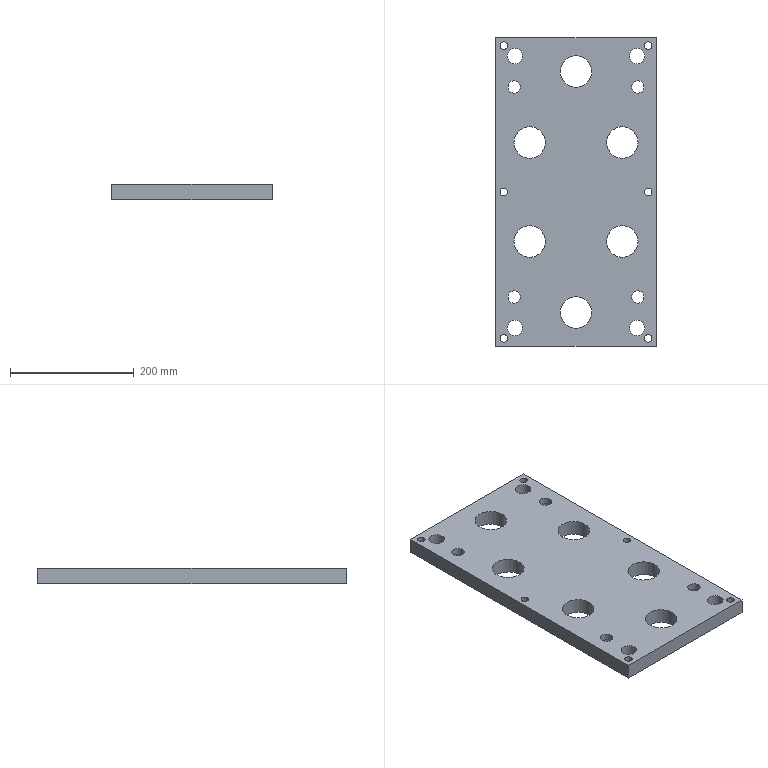Part | STEP file | SL2-MOLD_id702_xmt_txt | 1 solid | 42 faces | box 260 x 500 x 25 mm | volume 2824522 mm3 | cylinder 28 | plane 14 | commonest cylinder face diameters 12 x6 51 x6 20 x4 25 x4 28.5 x4 30 x4
STEP:
#1=CARTESIAN_POINT('',(49.5,170.,-214.));
#2=VERTEX_POINT('',#1);
#3=CARTESIAN_POINT('',(75.,170.,-214.));
#4=DIRECTION('',(0.,0.,-1.));
#5=DIRECTION('',(-1.,0.,0.));
#6=AXIS2_PLACEMENT_3D('',#3,#4,#5);
#7=CIRCLE('',#6,25.5);
#8=EDGE_CURVE('',#2,#2,#7,.T.);
#9=ORIENTED_EDGE('',*,*,#8,.F.);
#10=EDGE_LOOP('',(#9));
#11=FACE_BOUND('',#10,.T.);
#12=CARTESIAN_POINT('',(49.5,10.,-214.));
#13=VERTEX_POINT('',#12);
#14=CARTESIAN_POINT('',(75.,10.,-214.));
#15=DIRECTION('',(0.,0.,-1.));
#16=DIRECTION('',(-1.,0.,0.));
#17=AXIS2_PLACEMENT_3D('',#14,#15,#16);
#18=CIRCLE('',#17,25.5);
#19=EDGE_CURVE('',#13,#13,#18,.T.);
#20=ORIENTED_EDGE('',*,*,#19,.F.);
#21=EDGE_LOOP('',(#20));
#22=FACE_BOUND('',#21,.T.);
#23=CARTESIAN_POINT('',(-25.5,285.,-214.));
#24=VERTEX_POINT('',#23);
#25=CARTESIAN_POINT('',(0.,285.,-214.));
#26=DIRECTION('',(0.,0.,-1.));
#27=DIRECTION('',(-1.,0.,0.));
#28=AXIS2_PLACEMENT_3D('',#25,#26,#27);
#29=CIRCLE('',#28,25.5);
#30=EDGE_CURVE('',#24,#24,#29,.T.);
#31=ORIENTED_EDGE('',*,*,#30,.F.);
#32=EDGE_LOOP('',(#31));
#33=FACE_BOUND('',#32,.T.);
#34=CARTESIAN_POINT('',(-100.5,170.,-214.));
#35=VERTEX_POINT('',#34);
#36=CARTESIAN_POINT('',(-75.,170.,-214.));
#37=DIRECTION('',(0.,0.,-1.));
#38=DIRECTION('',(-1.,0.,0.));
#39=AXIS2_PLACEMENT_3D('',#36,#37,#38);
#40=CIRCLE('',#39,25.5);
#41=EDGE_CURVE('',#35,#35,#40,.T.);
#42=ORIENTED_EDGE('',*,*,#41,.F.);
#43=EDGE_LOOP('',(#42));
#44=FACE_BOUND('',#43,.T.);
#45=CARTESIAN_POINT('',(-25.5,-105.,-214.));
#46=VERTEX_POINT('',#45);
#47=CARTESIAN_POINT('',(0.,-105.,-214.));
#48=DIRECTION('',(0.,0.,-1.));
#49=DIRECTION('',(-1.,0.,0.));
#50=AXIS2_PLACEMENT_3D('',#47,#48,#49);
#51=CIRCLE('',#50,25.5);
#52=EDGE_CURVE('',#46,#46,#51,.T.);
#53=ORIENTED_EDGE('',*,*,#52,.F.);
#54=EDGE_LOOP('',(#53));
#55=FACE_BOUND('',#54,.T.);
#56=CARTESIAN_POINT('',(-100.5,10.,-214.));
#57=VERTEX_POINT('',#56);
#58=CARTESIAN_POINT('',(-75.,10.,-214.));
#59=DIRECTION('',(0.,0.,-1.));
#60=DIRECTION('',(-1.,0.,0.));
#61=AXIS2_PLACEMENT_3D('',#58,#59,#60);
#62=CIRCLE('',#61,25.5);
#63=EDGE_CURVE('',#57,#57,#62,.T.);
#64=ORIENTED_EDGE('',*,*,#63,.F.);
#65=EDGE_LOOP('',(#64));
#66=FACE_BOUND('',#65,.T.);
#67=CARTESIAN_POINT('',(-114.25,-80.,-214.));
#68=VERTEX_POINT('',#67);
#69=CARTESIAN_POINT('',(-100.,-80.,-214.));
#70=DIRECTION('',(0.,0.,1.));
#71=DIRECTION('',(-1.,0.,0.));
#72=AXIS2_PLACEMENT_3D('',#69,#70,#71);
#73=CIRCLE('',#72,14.25);
#74=EDGE_CURVE('',#68,#68,#73,.T.);
#75=ORIENTED_EDGE('',*,*,#74,.T.);
#76=EDGE_LOOP('',(#75));
#77=FACE_BOUND('',#76,.T.);
#78=CARTESIAN_POINT('',(85.75,-80.,-214.));
#79=VERTEX_POINT('',#78);
#80=CARTESIAN_POINT('',(100.,-80.,-214.));
#81=DIRECTION('',(0.,0.,1.));
#82=DIRECTION('',(-1.,0.,0.));
#83=AXIS2_PLACEMENT_3D('',#80,#81,#82);
#84=CIRCLE('',#83,14.25);
#85=EDGE_CURVE('',#79,#79,#84,.T.);
#86=ORIENTED_EDGE('',*,*,#85,.T.);
#87=EDGE_LOOP('',(#86));
#88=FACE_BOUND('',#87,.T.);
#89=CARTESIAN_POINT('',(85.75,260.,-214.));
#90=VERTEX_POINT('',#89);
#91=CARTESIAN_POINT('',(100.,260.,-214.));
#92=DIRECTION('',(0.,0.,1.));
#93=DIRECTION('',(-1.,0.,0.));
#94=AXIS2_PLACEMENT_3D('',#91,#92,#93);
#95=CIRCLE('',#94,14.25);
#96=EDGE_CURVE('',#90,#90,#95,.T.);
#97=ORIENTED_EDGE('',*,*,#96,.T.);
#98=EDGE_LOOP('',(#97));
#99=FACE_BOUND('',#98,.T.);
#100=CARTESIAN_POINT('',(-114.25,260.,-214.));
#101=VERTEX_POINT('',#100);
#102=CARTESIAN_POINT('',(-100.,260.,-214.));
#103=DIRECTION('',(0.,0.,1.));
#104=DIRECTION('',(-1.,0.,0.));
#105=AXIS2_PLACEMENT_3D('',#102,#103,#104);
#106=CIRCLE('',#105,14.25);
#107=EDGE_CURVE('',#101,#101,#106,.T.);
#108=ORIENTED_EDGE('',*,*,#107,.T.);
#109=EDGE_LOOP('',(#108));
#110=FACE_BOUND('',#109,.T.);
#111=CARTESIAN_POINT('',(-114.,310.,-214.));
#112=VERTEX_POINT('',#111);
#113=CARTESIAN_POINT('',(-99.,310.,-214.));
#114=DIRECTION('',(0.,0.,1.));
#115=DIRECTION('',(-1.,0.,0.));
#116=AXIS2_PLACEMENT_3D('',#113,#114,#115);
#117=CIRCLE('',#116,15.);
#118=EDGE_CURVE('',#112,#112,#117,.T.);
#119=ORIENTED_EDGE('',*,*,#118,.T.);
#120=EDGE_LOOP('',(#119));
#121=FACE_BOUND('',#120,.T.);
#122=CARTESIAN_POINT('',(84.,310.,-214.));
#123=VERTEX_POINT('',#122);
#124=CARTESIAN_POINT('',(99.,310.,-214.));
#125=DIRECTION('',(0.,0.,1.));
#126=DIRECTION('',(-1.,0.,0.));
#127=AXIS2_PLACEMENT_3D('',#124,#125,#126);
#128=CIRCLE('',#127,15.);
#129=EDGE_CURVE('',#123,#123,#128,.T.);
#130=ORIENTED_EDGE('',*,*,#129,.T.);
#131=EDGE_LOOP('',(#130));
#132=FACE_BOUND('',#131,.T.);
#133=CARTESIAN_POINT('',(84.,-130.,-214.));
#134=VERTEX_POINT('',#133);
#135=CARTESIAN_POINT('',(99.,-130.,-214.));
#136=DIRECTION('',(0.,0.,1.));
#137=DIRECTION('',(-1.,0.,0.));
#138=AXIS2_PLACEMENT_3D('',#135,#136,#137);
#139=CIRCLE('',#138,15.);
#140=EDGE_CURVE('',#134,#134,#139,.T.);
#141=ORIENTED_EDGE('',*,*,#140,.T.);
#142=EDGE_LOOP('',(#141));
#143=FACE_BOUND('',#142,.T.);
#144=CARTESIAN_POINT('',(-114.,-130.,-214.));
#145=VERTEX_POINT('',#144);
#146=CARTESIAN_POINT('',(-99.,-130.,-214.));
#147=DIRECTION('',(0.,0.,1.));
#148=DIRECTION('',(-1.,0.,0.));
#149=AXIS2_PLACEMENT_3D('',#146,#147,#148);
#150=CIRCLE('',#149,15.);
#151=EDGE_CURVE('',#145,#145,#150,.T.);
#152=ORIENTED_EDGE('',*,*,#151,.T.);
#153=EDGE_LOOP('',(#152));
#154=FACE_BOUND('',#153,.T.);
#155=CARTESIAN_POINT('',(111.,-147.,-214.));
#156=VERTEX_POINT('',#155);
#157=CARTESIAN_POINT('',(117.,-147.,-214.));
#158=DIRECTION('',(0.,0.,-1.));
#159=DIRECTION('',(-1.,0.,0.));
#160=AXIS2_PLACEMENT_3D('',#157,#158,#159);
#161=CIRCLE('',#160,6.);
#162=EDGE_CURVE('',#156,#156,#161,.T.);
#163=ORIENTED_EDGE('',*,*,#162,.F.);
#164=EDGE_LOOP('',(#163));
#165=FACE_BOUND('',#164,.T.);
#166=CARTESIAN_POINT('',(-123.,327.,-214.));
#167=VERTEX_POINT('',#166);
#168=CARTESIAN_POINT('',(-117.,327.,-214.));
#169=DIRECTION('',(0.,0.,-1.));
#170=DIRECTION('',(-1.,0.,0.));
#171=AXIS2_PLACEMENT_3D('',#168,#169,#170);
#172=CIRCLE('',#171,6.);
#173=EDGE_CURVE('',#167,#167,#172,.T.);
#174=ORIENTED_EDGE('',*,*,#173,.F.);
#175=EDGE_LOOP('',(#174));
#176=FACE_BOUND('',#175,.T.);
#177=CARTESIAN_POINT('',(-123.,-147.,-214.));
#178=VERTEX_POINT('',#177);
#179=CARTESIAN_POINT('',(-117.,-147.,-214.));
#180=DIRECTION('',(0.,0.,-1.));
#181=DIRECTION('',(-1.,0.,0.));
#182=AXIS2_PLACEMENT_3D('',#179,#180,#181);
#183=CIRCLE('',#182,6.);
#184=EDGE_CURVE('',#178,#178,#183,.T.);
#185=ORIENTED_EDGE('',*,*,#184,.F.);
#186=EDGE_LOOP('',(#185));
#187=FACE_BOUND('',#186,.T.);
#188=CARTESIAN_POINT('',(-123.,90.,-214.));
#189=VERTEX_POINT('',#188);
#190=CARTESIAN_POINT('',(-117.,90.,-214.));
#191=DIRECTION('',(0.,0.,-1.));
#192=DIRECTION('',(-1.,0.,0.));
#193=AXIS2_PLACEMENT_3D('',#190,#191,#192);
#194=CIRCLE('',#193,6.);
#195=EDGE_CURVE('',#189,#189,#194,.T.);
#196=ORIENTED_EDGE('',*,*,#195,.F.);
#197=EDGE_LOOP('',(#196));
#198=FACE_BOUND('',#197,.T.);
#199=CARTESIAN_POINT('',(111.,327.,-214.));
#200=VERTEX_POINT('',#199);
#201=CARTESIAN_POINT('',(117.,327.,-214.));
#202=DIRECTION('',(0.,0.,-1.));
#203=DIRECTION('',(-1.,0.,0.));
#204=AXIS2_PLACEMENT_3D('',#201,#202,#203);
#205=CIRCLE('',#204,6.);
#206=EDGE_CURVE('',#200,#200,#205,.T.);
#207=ORIENTED_EDGE('',*,*,#206,.F.);
#208=EDGE_LOOP('',(#207));
#209=FACE_BOUND('',#208,.T.);
#210=CARTESIAN_POINT('',(111.,90.,-214.));
#211=VERTEX_POINT('',#210);
#212=CARTESIAN_POINT('',(117.,90.,-214.));
#213=DIRECTION('',(0.,0.,-1.));
#214=DIRECTION('',(-1.,0.,0.));
#215=AXIS2_PLACEMENT_3D('',#212,#213,#214);
#216=CIRCLE('',#215,6.);
#217=EDGE_CURVE('',#211,#211,#216,.T.);
#218=ORIENTED_EDGE('',*,*,#217,.F.);
#219=EDGE_LOOP('',(#218));
#220=FACE_BOUND('',#219,.T.);
#221=CARTESIAN_POINT('',(-130.,-160.,-214.));
#222=VERTEX_POINT('',#221);
#223=CARTESIAN_POINT('',(130.,-160.,-214.));
#224=VERTEX_POINT('',#223);
#225=CARTESIAN_POINT('',(0.,-160.,-214.));
#226=DIRECTION('',(1.,0.,0.));
#227=VECTOR('',#226,1.);
#228=LINE('',#225,#227);
#229=EDGE_CURVE('',#222,#224,#228,.T.);
#230=ORIENTED_EDGE('',*,*,#229,.F.);
#231=CARTESIAN_POINT('',(-130.,340.,-214.));
#232=VERTEX_POINT('',#231);
#233=CARTESIAN_POINT('',(-130.,90.,-214.));
#234=DIRECTION('',(0.,1.,0.));
#235=VECTOR('',#234,1.);
#236=LINE('',#233,#235);
#237=EDGE_CURVE('',#222,#232,#236,.T.);
#238=ORIENTED_EDGE('',*,*,#237,.T.);
#239=CARTESIAN_POINT('',(130.,340.,-214.));
#240=VERTEX_POINT('',#239);
#241=CARTESIAN_POINT('',(0.,340.,-214.));
#242=DIRECTION('',(-1.,0.,0.));
#243=VECTOR('',#242,1.);
#244=LINE('',#241,#243);
#245=EDGE_CURVE('',#240,#232,#244,.T.);
#246=ORIENTED_EDGE('',*,*,#245,.F.);
#247=CARTESIAN_POINT('',(130.,90.,-214.));
#248=DIRECTION('',(0.,1.,0.));
#249=VECTOR('',#248,1.);
#250=LINE('',#247,#249);
#251=EDGE_CURVE('',#224,#240,#250,.T.);
#252=ORIENTED_EDGE('',*,*,#251,.F.);
#253=EDGE_LOOP('',(#230,#238,#246,#252));
#254=FACE_BOUND('',#253,.T.);
#255=CARTESIAN_POINT('',(0.,90.,-214.));
#256=DIRECTION('',(0.,0.,-1.));
#257=DIRECTION('',(-1.,0.,0.));
#258=AXIS2_PLACEMENT_3D('',#255,#256,#257);
#259=PLANE('',#258);
#260=ADVANCED_FACE('',(#11,#22,#33,#44,#55,#66,#77,#88,#99,#110,#121,#132,#143,#154,#165,#176,#187,#198,#209,#220,#254),#259,.T.);
#261=CARTESIAN_POINT('',(-130.,340.,-189.));
#262=VERTEX_POINT('',#261);
#263=CARTESIAN_POINT('',(130.,340.,-189.));
#264=VERTEX_POINT('',#263);
#265=CARTESIAN_POINT('',(0.,340.,-189.));
#266=DIRECTION('',(1.,0.,0.));
#267=VECTOR('',#266,1.);
#268=LINE('',#265,#267);
#269=EDGE_CURVE('',#262,#264,#268,.T.);
#270=ORIENTED_EDGE('',*,*,#269,.T.);
#271=CARTESIAN_POINT('',(130.,340.,-244.));
#272=DIRECTION('',(0.,0.,-1.));
#273=VECTOR('',#272,1.);
#274=LINE('',#271,#273);
#275=EDGE_CURVE('',#264,#240,#274,.T.);
#276=ORIENTED_EDGE('',*,*,#275,.T.);
#277=ORIENTED_EDGE('',*,*,#245,.T.);
#278=CARTESIAN_POINT('',(-130.,340.,-244.));
#279=DIRECTION('',(0.,0.,1.));
#280=VECTOR('',#279,1.);
#281=LINE('',#278,#280);
#282=EDGE_CURVE('',#232,#262,#281,.T.);
#283=ORIENTED_EDGE('',*,*,#282,.T.);
#284=EDGE_LOOP('',(#270,#276,#277,#283));
#285=FACE_OUTER_BOUND('',#284,.T.);
#286=CARTESIAN_POINT('',(0.,340.,-244.));
#287=DIRECTION('',(0.,1.,0.));
#288=DIRECTION('',(0.,0.,1.));
#289=AXIS2_PLACEMENT_3D('',#286,#287,#288);
#290=PLANE('',#289);
#291=ADVANCED_FACE('',(#285),#290,.T.);
#292=CARTESIAN_POINT('',(-130.,-160.,-189.));
#293=VERTEX_POINT('',#292);
#294=CARTESIAN_POINT('',(130.,-160.,-189.));
#295=VERTEX_POINT('',#294);
#296=CARTESIAN_POINT('',(0.,-160.,-189.));
#297=DIRECTION('',(1.,0.,0.));
#298=VECTOR('',#297,1.);
#299=LINE('',#296,#298);
#300=EDGE_CURVE('',#293,#295,#299,.T.);
#301=ORIENTED_EDGE('',*,*,#300,.F.);
#302=CARTESIAN_POINT('',(-130.,-160.,-244.));
#303=DIRECTION('',(0.,0.,-1.));
#304=VECTOR('',#303,1.);
#305=LINE('',#302,#304);
#306=EDGE_CURVE('',#293,#222,#305,.T.);
#307=ORIENTED_EDGE('',*,*,#306,.T.);
#308=ORIENTED_EDGE('',*,*,#229,.T.);
#309=CARTESIAN_POINT('',(130.,-160.,-179.));
#310=DIRECTION('',(0.,0.,-1.));
#311=VECTOR('',#310,1.);
#312=LINE('',#309,#311);
#313=EDGE_CURVE('',#295,#224,#312,.T.);
#314=ORIENTED_EDGE('',*,*,#313,.F.);
#315=EDGE_LOOP('',(#301,#307,#308,#314));
#316=FACE_OUTER_BOUND('',#315,.T.);
#317=CARTESIAN_POINT('',(0.,-160.,-244.));
#318=DIRECTION('',(0.,-1.,0.));
#319=DIRECTION('',(0.,0.,-1.));
#320=AXIS2_PLACEMENT_3D('',#317,#318,#319);
#321=PLANE('',#320);
#322=ADVANCED_FACE('',(#316),#321,.T.);
#323=CARTESIAN_POINT('',(130.,90.,-189.));
#324=DIRECTION('',(0.,1.,0.));
#325=VECTOR('',#324,1.);
#326=LINE('',#323,#325);
#327=EDGE_CURVE('',#295,#264,#326,.T.);
#328=ORIENTED_EDGE('',*,*,#327,.F.);
#329=ORIENTED_EDGE('',*,*,#313,.T.);
#330=ORIENTED_EDGE('',*,*,#251,.T.);
#331=ORIENTED_EDGE('',*,*,#275,.F.);
#332=EDGE_LOOP('',(#328,#329,#330,#331));
#333=FACE_OUTER_BOUND('',#332,.T.);
#334=CARTESIAN_POINT('',(130.,90.,-179.));
#335=DIRECTION('',(1.,0.,0.));
#336=DIRECTION('',(0.,0.,-1.));
#337=AXIS2_PLACEMENT_3D('',#334,#335,#336);
#338=PLANE('',#337);
#339=ADVANCED_FACE('',(#333),#338,.T.);
#340=CARTESIAN_POINT('',(-130.,90.,-189.));
#341=DIRECTION('',(0.,-1.,0.));
#342=VECTOR('',#341,1.);
#343=LINE('',#340,#342);
#344=EDGE_CURVE('',#262,#293,#343,.T.);
#345=ORIENTED_EDGE('',*,*,#344,.F.);
#346=ORIENTED_EDGE('',*,*,#282,.F.);
#347=ORIENTED_EDGE('',*,*,#237,.F.);
#348=ORIENTED_EDGE('',*,*,#306,.F.);
#349=EDGE_LOOP('',(#345,#346,#347,#348));
#350=FACE_OUTER_BOUND('',#349,.T.);
#351=CARTESIAN_POINT('',(-130.,90.,-179.));
#352=DIRECTION('',(-1.,0.,0.));
#353=DIRECTION('',(0.,0.,1.));
#354=AXIS2_PLACEMENT_3D('',#351,#352,#353);
#355=PLANE('',#354);
#356=ADVANCED_FACE('',(#350),#355,.T.);
#357=CARTESIAN_POINT('',(49.5,170.,-189.));
#358=VERTEX_POINT('',#357);
#359=CARTESIAN_POINT('',(75.,170.,-189.));
#360=DIRECTION('',(0.,0.,-1.));
#361=DIRECTION('',(-1.,0.,0.));
#362=AXIS2_PLACEMENT_3D('',#359,#360,#361);
#363=CIRCLE('',#362,25.5);
#364=EDGE_CURVE('',#358,#358,#363,.T.);
#365=ORIENTED_EDGE('',*,*,#364,.T.);
#366=EDGE_LOOP('',(#365));
#367=FACE_BOUND('',#366,.T.);
#368=CARTESIAN_POINT('',(49.5,10.,-189.));
#369=VERTEX_POINT('',#368);
#370=CARTESIAN_POINT('',(75.,10.,-189.));
#371=DIRECTION('',(0.,0.,-1.));
#372=DIRECTION('',(-1.,0.,0.));
#373=AXIS2_PLACEMENT_3D('',#370,#371,#372);
#374=CIRCLE('',#373,25.5);
#375=EDGE_CURVE('',#369,#369,#374,.T.);
#376=ORIENTED_EDGE('',*,*,#375,.T.);
#377=EDGE_LOOP('',(#376));
#378=FACE_BOUND('',#377,.T.);
#379=CARTESIAN_POINT('',(-25.5,285.,-189.));
#380=VERTEX_POINT('',#379);
#381=CARTESIAN_POINT('',(0.,285.,-189.));
#382=DIRECTION('',(0.,0.,-1.));
#383=DIRECTION('',(-1.,0.,0.));
#384=AXIS2_PLACEMENT_3D('',#381,#382,#383);
#385=CIRCLE('',#384,25.5);
#386=EDGE_CURVE('',#380,#380,#385,.T.);
#387=ORIENTED_EDGE('',*,*,#386,.T.);
#388=EDGE_LOOP('',(#387));
#389=FACE_BOUND('',#388,.T.);
#390=CARTESIAN_POINT('',(-100.5,170.,-189.));
#391=VERTEX_POINT('',#390);
#392=CARTESIAN_POINT('',(-75.,170.,-189.));
#393=DIRECTION('',(0.,0.,-1.));
#394=DIRECTION('',(-1.,0.,0.));
#395=AXIS2_PLACEMENT_3D('',#392,#393,#394);
#396=CIRCLE('',#395,25.5);
#397=EDGE_CURVE('',#391,#391,#396,.T.);
#398=ORIENTED_EDGE('',*,*,#397,.T.);
#399=EDGE_LOOP('',(#398));
#400=FACE_BOUND('',#399,.T.);
#401=CARTESIAN_POINT('',(-25.5,-105.,-189.));
#402=VERTEX_POINT('',#401);
#403=CARTESIAN_POINT('',(0.,-105.,-189.));
#404=DIRECTION('',(0.,0.,-1.));
#405=DIRECTION('',(-1.,0.,0.));
#406=AXIS2_PLACEMENT_3D('',#403,#404,#405);
#407=CIRCLE('',#406,25.5);
#408=EDGE_CURVE('',#402,#402,#407,.T.);
#409=ORIENTED_EDGE('',*,*,#408,.T.);
#410=EDGE_LOOP('',(#409));
#411=FACE_BOUND('',#410,.T.);
#412=CARTESIAN_POINT('',(-100.5,10.,-189.));
#413=VERTEX_POINT('',#412);
#414=CARTESIAN_POINT('',(-75.,10.,-189.));
#415=DIRECTION('',(0.,0.,-1.));
#416=DIRECTION('',(-1.,0.,0.));
#417=AXIS2_PLACEMENT_3D('',#414,#415,#416);
#418=CIRCLE('',#417,25.5);
#419=EDGE_CURVE('',#413,#413,#418,.T.);
#420=ORIENTED_EDGE('',*,*,#419,.T.);
#421=EDGE_LOOP('',(#420));
#422=FACE_BOUND('',#421,.T.);
#423=CARTESIAN_POINT('',(90.,260.,-189.));
#424=VERTEX_POINT('',#423);
#425=CARTESIAN_POINT('',(100.,260.,-189.));
#426=DIRECTION('',(0.,0.,1.));
#427=DIRECTION('',(-1.,0.,0.));
#428=AXIS2_PLACEMENT_3D('',#425,#426,#427);
#429=CIRCLE('',#428,10.);
#430=EDGE_CURVE('',#424,#424,#429,.T.);
#431=ORIENTED_EDGE('',*,*,#430,.F.);
#432=EDGE_LOOP('',(#431));
#433=FACE_BOUND('',#432,.T.);
#434=CARTESIAN_POINT('',(90.,-80.,-189.));
#435=VERTEX_POINT('',#434);
#436=CARTESIAN_POINT('',(100.,-80.,-189.));
#437=DIRECTION('',(0.,0.,1.));
#438=DIRECTION('',(-1.,0.,0.));
#439=AXIS2_PLACEMENT_3D('',#436,#437,#438);
#440=CIRCLE('',#439,10.);
#441=EDGE_CURVE('',#435,#435,#440,.T.);
#442=ORIENTED_EDGE('',*,*,#441,.F.);
#443=EDGE_LOOP('',(#442));
#444=FACE_BOUND('',#443,.T.);
#445=CARTESIAN_POINT('',(-110.,-80.,-189.));
#446=VERTEX_POINT('',#445);
#447=CARTESIAN_POINT('',(-100.,-80.,-189.));
#448=DIRECTION('',(0.,0.,1.));
#449=DIRECTION('',(-1.,0.,0.));
#450=AXIS2_PLACEMENT_3D('',#447,#448,#449);
#451=CIRCLE('',#450,10.);
#452=EDGE_CURVE('',#446,#446,#451,.T.);
#453=ORIENTED_EDGE('',*,*,#452,.F.);
#454=EDGE_LOOP('',(#453));
#455=FACE_BOUND('',#454,.T.);
#456=CARTESIAN_POINT('',(-110.,260.,-189.));
#457=VERTEX_POINT('',#456);
#458=CARTESIAN_POINT('',(-100.,260.,-189.));
#459=DIRECTION('',(0.,0.,1.));
#460=DIRECTION('',(-1.,0.,0.));
#461=AXIS2_PLACEMENT_3D('',#458,#459,#460);
#462=CIRCLE('',#461,10.);
#463=EDGE_CURVE('',#457,#457,#462,.T.);
#464=ORIENTED_EDGE('',*,*,#463,.F.);
#465=EDGE_LOOP('',(#464));
#466=FACE_BOUND('',#465,.T.);
#467=CARTESIAN_POINT('',(86.5,310.,-189.));
#468=VERTEX_POINT('',#467);
#469=CARTESIAN_POINT('',(99.,310.,-189.));
#470=DIRECTION('',(0.,0.,1.));
#471=DIRECTION('',(-1.,0.,0.));
#472=AXIS2_PLACEMENT_3D('',#469,#470,#471);
#473=CIRCLE('',#472,12.5);
#474=EDGE_CURVE('',#468,#468,#473,.T.);
#475=ORIENTED_EDGE('',*,*,#474,.F.);
#476=EDGE_LOOP('',(#475));
#477=FACE_BOUND('',#476,.T.);
#478=CARTESIAN_POINT('',(-111.5,310.,-189.));
#479=VERTEX_POINT('',#478);
#480=CARTESIAN_POINT('',(-99.,310.,-189.));
#481=DIRECTION('',(0.,0.,1.));
#482=DIRECTION('',(-1.,0.,0.));
#483=AXIS2_PLACEMENT_3D('',#480,#481,#482);
#484=CIRCLE('',#483,12.5);
#485=EDGE_CURVE('',#479,#479,#484,.T.);
#486=ORIENTED_EDGE('',*,*,#485,.F.);
#487=EDGE_LOOP('',(#486));
#488=FACE_BOUND('',#487,.T.);
#489=CARTESIAN_POINT('',(86.5,-130.,-189.));
#490=VERTEX_POINT('',#489);
#491=CARTESIAN_POINT('',(99.,-130.,-189.));
#492=DIRECTION('',(0.,0.,1.));
#493=DIRECTION('',(-1.,0.,0.));
#494=AXIS2_PLACEMENT_3D('',#491,#492,#493);
#495=CIRCLE('',#494,12.5);
#496=EDGE_CURVE('',#490,#490,#495,.T.);
#497=ORIENTED_EDGE('',*,*,#496,.F.);
#498=EDGE_LOOP('',(#497));
#499=FACE_BOUND('',#498,.T.);
#500=CARTESIAN_POINT('',(-111.5,-130.,-189.));
#501=VERTEX_POINT('',#500);
#502=CARTESIAN_POINT('',(-99.,-130.,-189.));
#503=DIRECTION('',(0.,0.,1.));
#504=DIRECTION('',(-1.,0.,0.));
#505=AXIS2_PLACEMENT_3D('',#502,#503,#504);
#506=CIRCLE('',#505,12.5);
#507=EDGE_CURVE('',#501,#501,#506,.T.);
#508=ORIENTED_EDGE('',*,*,#507,.F.);
#509=EDGE_LOOP('',(#508));
#510=FACE_BOUND('',#509,.T.);
#511=CARTESIAN_POINT('',(111.,-147.,-189.));
#512=VERTEX_POINT('',#511);
#513=CARTESIAN_POINT('',(117.,-147.,-189.));
#514=DIRECTION('',(0.,0.,-1.));
#515=DIRECTION('',(-1.,0.,0.));
#516=AXIS2_PLACEMENT_3D('',#513,#514,#515);
#517=CIRCLE('',#516,6.);
#518=EDGE_CURVE('',#512,#512,#517,.T.);
#519=ORIENTED_EDGE('',*,*,#518,.T.);
#520=EDGE_LOOP('',(#519));
#521=FACE_BOUND('',#520,.T.);
#522=CARTESIAN_POINT('',(-123.,327.,-189.));
#523=VERTEX_POINT('',#522);
#524=CARTESIAN_POINT('',(-117.,327.,-189.));
#525=DIRECTION('',(0.,0.,-1.));
#526=DIRECTION('',(-1.,0.,0.));
#527=AXIS2_PLACEMENT_3D('',#524,#525,#526);
#528=CIRCLE('',#527,6.);
#529=EDGE_CURVE('',#523,#523,#528,.T.);
#530=ORIENTED_EDGE('',*,*,#529,.T.);
#531=EDGE_LOOP('',(#530));
#532=FACE_BOUND('',#531,.T.);
#533=CARTESIAN_POINT('',(-123.,-147.,-189.));
#534=VERTEX_POINT('',#533);
#535=CARTESIAN_POINT('',(-117.,-147.,-189.));
#536=DIRECTION('',(0.,0.,-1.));
#537=DIRECTION('',(-1.,0.,0.));
#538=AXIS2_PLACEMENT_3D('',#535,#536,#537);
#539=CIRCLE('',#538,6.);
#540=EDGE_CURVE('',#534,#534,#539,.T.);
#541=ORIENTED_EDGE('',*,*,#540,.T.);
#542=EDGE_LOOP('',(#541));
#543=FACE_BOUND('',#542,.T.);
#544=CARTESIAN_POINT('',(-123.,90.,-189.));
#545=VERTEX_POINT('',#544);
#546=CARTESIAN_POINT('',(-117.,90.,-189.));
#547=DIRECTION('',(0.,0.,-1.));
#548=DIRECTION('',(-1.,0.,0.));
#549=AXIS2_PLACEMENT_3D('',#546,#547,#548);
#550=CIRCLE('',#549,6.);
#551=EDGE_CURVE('',#545,#545,#550,.T.);
#552=ORIENTED_EDGE('',*,*,#551,.T.);
#553=EDGE_LOOP('',(#552));
#554=FACE_BOUND('',#553,.T.);
#555=CARTESIAN_POINT('',(111.,327.,-189.));
#556=VERTEX_POINT('',#555);
#557=CARTESIAN_POINT('',(117.,327.,-189.));
#558=DIRECTION('',(0.,0.,-1.));
#559=DIRECTION('',(-1.,0.,0.));
#560=AXIS2_PLACEMENT_3D('',#557,#558,#559);
#561=CIRCLE('',#560,6.);
#562=EDGE_CURVE('',#556,#556,#561,.T.);
#563=ORIENTED_EDGE('',*,*,#562,.T.);
#564=EDGE_LOOP('',(#563));
#565=FACE_BOUND('',#564,.T.);
#566=CARTESIAN_POINT('',(111.,90.,-189.));
#567=VERTEX_POINT('',#566);
#568=CARTESIAN_POINT('',(117.,90.,-189.));
#569=DIRECTION('',(0.,0.,-1.));
#570=DIRECTION('',(-1.,0.,0.));
#571=AXIS2_PLACEMENT_3D('',#568,#569,#570);
#572=CIRCLE('',#571,6.);
#573=EDGE_CURVE('',#567,#567,#572,.T.);
#574=ORIENTED_EDGE('',*,*,#573,.T.);
#575=EDGE_LOOP('',(#574));
#576=FACE_BOUND('',#575,.T.);
#577=ORIENTED_EDGE('',*,*,#327,.T.);
#578=ORIENTED_EDGE('',*,*,#269,.F.);
#579=ORIENTED_EDGE('',*,*,#344,.T.);
#580=ORIENTED_EDGE('',*,*,#300,.T.);
#581=EDGE_LOOP('',(#577,#578,#579,#580));
#582=FACE_BOUND('',#581,.T.);
#583=CARTESIAN_POINT('',(0.,90.,-189.));
#584=DIRECTION('',(0.,0.,-1.));
#585=DIRECTION('',(-1.,0.,0.));
#586=AXIS2_PLACEMENT_3D('',#583,#584,#585);
#587=PLANE('',#586);
#588=ADVANCED_FACE('',(#367,#378,#389,#400,#411,#422,#433,#444,#455,#466,#477,#488,#499,#510,#521,#532,#543,#554,#565,#576,#582),#587,.F.);
#589=ORIENTED_EDGE('',*,*,#217,.T.);
#590=EDGE_LOOP('',(#589));
#591=FACE_BOUND('',#590,.T.);
#592=ORIENTED_EDGE('',*,*,#573,.F.);
#593=EDGE_LOOP('',(#592));
#594=FACE_BOUND('',#593,.T.);
#595=CARTESIAN_POINT('',(117.,90.,263.));
#596=DIRECTION('',(0.,0.,-1.));
#597=DIRECTION('',(-1.,0.,0.));
#598=AXIS2_PLACEMENT_3D('',#595,#596,#597);
#599=CYLINDRICAL_SURFACE('',#598,6.);
#600=ADVANCED_FACE('',(#591,#594),#599,.F.);
#601=ORIENTED_EDGE('',*,*,#206,.T.);
#602=EDGE_LOOP('',(#601));
#603=FACE_BOUND('',#602,.T.);
#604=ORIENTED_EDGE('',*,*,#562,.F.);
#605=EDGE_LOOP('',(#604));
#606=FACE_BOUND('',#605,.T.);
#607=CARTESIAN_POINT('',(117.,327.,263.));
#608=DIRECTION('',(0.,0.,-1.));
#609=DIRECTION('',(-1.,0.,0.));
#610=AXIS2_PLACEMENT_3D('',#607,#608,#609);
#611=CYLINDRICAL_SURFACE('',#610,6.);
#612=ADVANCED_FACE('',(#603,#606),#611,.F.);
#613=ORIENTED_EDGE('',*,*,#195,.T.);
#614=EDGE_LOOP('',(#613));
#615=FACE_BOUND('',#614,.T.);
#616=ORIENTED_EDGE('',*,*,#551,.F.);
#617=EDGE_LOOP('',(#616));
#618=FACE_BOUND('',#617,.T.);
#619=CARTESIAN_POINT('',(-117.,90.,263.));
#620=DIRECTION('',(0.,0.,-1.));
#621=DIRECTION('',(-1.,0.,0.));
#622=AXIS2_PLACEMENT_3D('',#619,#620,#621);
#623=CYLINDRICAL_SURFACE('',#622,6.);
#624=ADVANCED_FACE('',(#615,#618),#623,.F.);
#625=ORIENTED_EDGE('',*,*,#184,.T.);
#626=EDGE_LOOP('',(#625));
#627=FACE_BOUND('',#626,.T.);
#628=ORIENTED_EDGE('',*,*,#540,.F.);
#629=EDGE_LOOP('',(#628));
#630=FACE_BOUND('',#629,.T.);
#631=CARTESIAN_POINT('',(-117.,-147.,263.));
#632=DIRECTION('',(0.,0.,-1.));
#633=DIRECTION('',(-1.,0.,0.));
#634=AXIS2_PLACEMENT_3D('',#631,#632,#633);
#635=CYLINDRICAL_SURFACE('',#634,6.);
#636=ADVANCED_FACE('',(#627,#630),#635,.F.);
#637=ORIENTED_EDGE('',*,*,#173,.T.);
#638=EDGE_LOOP('',(#637));
#639=FACE_BOUND('',#638,.T.);
#640=ORIENTED_EDGE('',*,*,#529,.F.);
#641=EDGE_LOOP('',(#640));
#642=FACE_BOUND('',#641,.T.);
#643=CARTESIAN_POINT('',(-117.,327.,263.));
#644=DIRECTION('',(0.,0.,-1.));
#645=DIRECTION('',(-1.,0.,0.));
#646=AXIS2_PLACEMENT_3D('',#643,#644,#645);
#647=CYLINDRICAL_SURFACE('',#646,6.);
#648=ADVANCED_FACE('',(#639,#642),#647,.F.);
#649=ORIENTED_EDGE('',*,*,#162,.T.);
#650=EDGE_LOOP('',(#649));
#651=FACE_BOUND('',#650,.T.);
#652=ORIENTED_EDGE('',*,*,#518,.F.);
#653=EDGE_LOOP('',(#652));
#654=FACE_BOUND('',#653,.T.);
#655=CARTESIAN_POINT('',(117.,-147.,263.));
#656=DIRECTION('',(0.,0.,-1.));
#657=DIRECTION('',(-1.,0.,0.));
#658=AXIS2_PLACEMENT_3D('',#655,#656,#657);
#659=CYLINDRICAL_SURFACE('',#658,6.);
#660=ADVANCED_FACE('',(#651,#654),#659,.F.);
#661=ORIENTED_EDGE('',*,*,#151,.F.);
#662=EDGE_LOOP('',(#661));
#663=FACE_BOUND('',#662,.T.);
#664=CARTESIAN_POINT('',(-84.,-130.,-210.));
#665=VERTEX_POINT('',#664);
#666=CARTESIAN_POINT('',(-99.,-130.,-210.));
#667=DIRECTION('',(0.,0.,1.));
#668=DIRECTION('',(1.,0.,0.));
#669=AXIS2_PLACEMENT_3D('',#666,#667,#668);
#670=CIRCLE('',#669,15.);
#671=EDGE_CURVE('',#665,#665,#670,.T.);
#672=ORIENTED_EDGE('',*,*,#671,.T.);
#673=EDGE_LOOP('',(#672));
#674=FACE_BOUND('',#673,.T.);
#675=CARTESIAN_POINT('',(-99.,-130.,-240.));
#676=DIRECTION('',(0.,0.,1.));
#677=DIRECTION('',(1.,0.,0.));
#678=AXIS2_PLACEMENT_3D('',#675,#676,#677);
#679=CYLINDRICAL_SURFACE('',#678,15.);
#680=ADVANCED_FACE('',(#663,#674),#679,.F.);
#681=CARTESIAN_POINT('',(-86.5,-130.,-210.));
#682=VERTEX_POINT('',#681);
#683=CARTESIAN_POINT('',(-99.,-130.,-210.));
#684=DIRECTION('',(0.,0.,1.));
#685=DIRECTION('',(1.,0.,0.));
#686=AXIS2_PLACEMENT_3D('',#683,#684,#685);
#687=CIRCLE('',#686,12.5);
#688=EDGE_CURVE('',#682,#682,#687,.T.);
#689=ORIENTED_EDGE('',*,*,#688,.T.);
#690=EDGE_LOOP('',(#689));
#691=FACE_BOUND('',#690,.T.);
#692=ORIENTED_EDGE('',*,*,#671,.F.);
#693=EDGE_LOOP('',(#692));
#694=FACE_BOUND('',#693,.T.);
#695=CARTESIAN_POINT('',(-99.,-130.,-210.));
#696=DIRECTION('',(0.,0.,-1.));
#697=DIRECTION('',(-1.,0.,0.));
#698=AXIS2_PLACEMENT_3D('',#695,#696,#697);
#699=PLANE('',#698);
#700=ADVANCED_FACE('',(#691,#694),#699,.T.);
#701=ORIENTED_EDGE('',*,*,#140,.F.);
#702=EDGE_LOOP('',(#701));
#703=FACE_BOUND('',#702,.T.);
#704=CARTESIAN_POINT('',(114.,-130.,-210.));
#705=VERTEX_POINT('',#704);
#706=CARTESIAN_POINT('',(99.,-130.,-210.));
#707=DIRECTION('',(0.,0.,1.));
#708=DIRECTION('',(1.,0.,0.));
#709=AXIS2_PLACEMENT_3D('',#706,#707,#708);
#710=CIRCLE('',#709,15.);
#711=EDGE_CURVE('',#705,#705,#710,.T.);
#712=ORIENTED_EDGE('',*,*,#711,.T.);
#713=EDGE_LOOP('',(#712));
#714=FACE_BOUND('',#713,.T.);
#715=CARTESIAN_POINT('',(99.,-130.,-240.));
#716=DIRECTION('',(0.,0.,1.));
#717=DIRECTION('',(1.,0.,0.));
#718=AXIS2_PLACEMENT_3D('',#715,#716,#717);
#719=CYLINDRICAL_SURFACE('',#718,15.);
#720=ADVANCED_FACE('',(#703,#714),#719,.F.);
#721=CARTESIAN_POINT('',(111.5,-130.,-210.));
#722=VERTEX_POINT('',#721);
#723=CARTESIAN_POINT('',(99.,-130.,-210.));
#724=DIRECTION('',(0.,0.,1.));
#725=DIRECTION('',(1.,0.,0.));
#726=AXIS2_PLACEMENT_3D('',#723,#724,#725);
#727=CIRCLE('',#726,12.5);
#728=EDGE_CURVE('',#722,#722,#727,.T.);
#729=ORIENTED_EDGE('',*,*,#728,.T.);
#730=EDGE_LOOP('',(#729));
#731=FACE_BOUND('',#730,.T.);
#732=ORIENTED_EDGE('',*,*,#711,.F.);
#733=EDGE_LOOP('',(#732));
#734=FACE_BOUND('',#733,.T.);
#735=CARTESIAN_POINT('',(99.,-130.,-210.));
#736=DIRECTION('',(0.,0.,-1.));
#737=DIRECTION('',(-1.,0.,0.));
#738=AXIS2_PLACEMENT_3D('',#735,#736,#737);
#739=PLANE('',#738);
#740=ADVANCED_FACE('',(#731,#734),#739,.T.);
#741=ORIENTED_EDGE('',*,*,#129,.F.);
#742=EDGE_LOOP('',(#741));
#743=FACE_BOUND('',#742,.T.);
#744=CARTESIAN_POINT('',(114.,310.,-210.));
#745=VERTEX_POINT('',#744);
#746=CARTESIAN_POINT('',(99.,310.,-210.));
#747=DIRECTION('',(0.,0.,1.));
#748=DIRECTION('',(1.,0.,0.));
#749=AXIS2_PLACEMENT_3D('',#746,#747,#748);
#750=CIRCLE('',#749,15.);
#751=EDGE_CURVE('',#745,#745,#750,.T.);
#752=ORIENTED_EDGE('',*,*,#751,.T.);
#753=EDGE_LOOP('',(#752));
#754=FACE_BOUND('',#753,.T.);
#755=CARTESIAN_POINT('',(99.,310.,-240.));
#756=DIRECTION('',(0.,0.,1.));
#757=DIRECTION('',(1.,0.,0.));
#758=AXIS2_PLACEMENT_3D('',#755,#756,#757);
#759=CYLINDRICAL_SURFACE('',#758,15.);
#760=ADVANCED_FACE('',(#743,#754),#759,.F.);
#761=CARTESIAN_POINT('',(111.5,310.,-210.));
#762=VERTEX_POINT('',#761);
#763=CARTESIAN_POINT('',(99.,310.,-210.));
#764=DIRECTION('',(0.,0.,1.));
#765=DIRECTION('',(1.,0.,0.));
#766=AXIS2_PLACEMENT_3D('',#763,#764,#765);
#767=CIRCLE('',#766,12.5);
#768=EDGE_CURVE('',#762,#762,#767,.T.);
#769=ORIENTED_EDGE('',*,*,#768,.T.);
#770=EDGE_LOOP('',(#769));
#771=FACE_BOUND('',#770,.T.);
#772=ORIENTED_EDGE('',*,*,#751,.F.);
#773=EDGE_LOOP('',(#772));
#774=FACE_BOUND('',#773,.T.);
#775=CARTESIAN_POINT('',(99.,310.,-210.));
#776=DIRECTION('',(0.,0.,-1.));
#777=DIRECTION('',(-1.,0.,0.));
#778=AXIS2_PLACEMENT_3D('',#775,#776,#777);
#779=PLANE('',#778);
#780=ADVANCED_FACE('',(#771,#774),#779,.T.);
#781=ORIENTED_EDGE('',*,*,#118,.F.);
#782=EDGE_LOOP('',(#781));
#783=FACE_BOUND('',#782,.T.);
#784=CARTESIAN_POINT('',(-84.,310.,-210.));
#785=VERTEX_POINT('',#784);
#786=CARTESIAN_POINT('',(-99.,310.,-210.));
#787=DIRECTION('',(0.,0.,1.));
#788=DIRECTION('',(1.,0.,0.));
#789=AXIS2_PLACEMENT_3D('',#786,#787,#788);
#790=CIRCLE('',#789,15.);
#791=EDGE_CURVE('',#785,#785,#790,.T.);
#792=ORIENTED_EDGE('',*,*,#791,.T.);
#793=EDGE_LOOP('',(#792));
#794=FACE_BOUND('',#793,.T.);
#795=CARTESIAN_POINT('',(-99.,310.,-240.));
#796=DIRECTION('',(0.,0.,1.));
#797=DIRECTION('',(1.,0.,0.));
#798=AXIS2_PLACEMENT_3D('',#795,#796,#797);
#799=CYLINDRICAL_SURFACE('',#798,15.);
#800=ADVANCED_FACE('',(#783,#794),#799,.F.);
#801=CARTESIAN_POINT('',(-86.5,310.,-210.));
#802=VERTEX_POINT('',#801);
#803=CARTESIAN_POINT('',(-99.,310.,-210.));
#804=DIRECTION('',(0.,0.,1.));
#805=DIRECTION('',(1.,0.,0.));
#806=AXIS2_PLACEMENT_3D('',#803,#804,#805);
#807=CIRCLE('',#806,12.5);
#808=EDGE_CURVE('',#802,#802,#807,.T.);
#809=ORIENTED_EDGE('',*,*,#808,.T.);
#810=EDGE_LOOP('',(#809));
#811=FACE_BOUND('',#810,.T.);
#812=ORIENTED_EDGE('',*,*,#791,.F.);
#813=EDGE_LOOP('',(#812));
#814=FACE_BOUND('',#813,.T.);
#815=CARTESIAN_POINT('',(-99.,310.,-210.));
#816=DIRECTION('',(0.,0.,-1.));
#817=DIRECTION('',(-1.,0.,0.));
#818=AXIS2_PLACEMENT_3D('',#815,#816,#817);
#819=PLANE('',#818);
#820=ADVANCED_FACE('',(#811,#814),#819,.T.);
#821=ORIENTED_EDGE('',*,*,#688,.F.);
#822=EDGE_LOOP('',(#821));
#823=FACE_BOUND('',#822,.T.);
#824=ORIENTED_EDGE('',*,*,#507,.T.);
#825=EDGE_LOOP('',(#824));
#826=FACE_BOUND('',#825,.T.);
#827=CARTESIAN_POINT('',(-99.,-130.,-2221.4));
#828=DIRECTION('',(0.,0.,1.));
#829=DIRECTION('',(1.,0.,0.));
#830=AXIS2_PLACEMENT_3D('',#827,#828,#829);
#831=CYLINDRICAL_SURFACE('',#830,12.5);
#832=ADVANCED_FACE('',(#823,#826),#831,.F.);
#833=ORIENTED_EDGE('',*,*,#728,.F.);
#834=EDGE_LOOP('',(#833));
#835=FACE_BOUND('',#834,.T.);
#836=ORIENTED_EDGE('',*,*,#496,.T.);
#837=EDGE_LOOP('',(#836));
#838=FACE_BOUND('',#837,.T.);
#839=CARTESIAN_POINT('',(99.,-130.,-2221.4));
#840=DIRECTION('',(0.,0.,1.));
#841=DIRECTION('',(1.,0.,0.));
#842=AXIS2_PLACEMENT_3D('',#839,#840,#841);
#843=CYLINDRICAL_SURFACE('',#842,12.5);
#844=ADVANCED_FACE('',(#835,#838),#843,.F.);
#845=ORIENTED_EDGE('',*,*,#808,.F.);
#846=EDGE_LOOP('',(#845));
#847=FACE_BOUND('',#846,.T.);
#848=ORIENTED_EDGE('',*,*,#485,.T.);
#849=EDGE_LOOP('',(#848));
#850=FACE_BOUND('',#849,.T.);
#851=CARTESIAN_POINT('',(-99.,310.,-2221.4));
#852=DIRECTION('',(0.,0.,1.));
#853=DIRECTION('',(1.,0.,0.));
#854=AXIS2_PLACEMENT_3D('',#851,#852,#853);
#855=CYLINDRICAL_SURFACE('',#854,12.5);
#856=ADVANCED_FACE('',(#847,#850),#855,.F.);
#857=ORIENTED_EDGE('',*,*,#768,.F.);
#858=EDGE_LOOP('',(#857));
#859=FACE_BOUND('',#858,.T.);
#860=ORIENTED_EDGE('',*,*,#474,.T.);
#861=EDGE_LOOP('',(#860));
#862=FACE_BOUND('',#861,.T.);
#863=CARTESIAN_POINT('',(99.,310.,-2221.4));
#864=DIRECTION('',(0.,0.,1.));
#865=DIRECTION('',(1.,0.,0.));
#866=AXIS2_PLACEMENT_3D('',#863,#864,#865);
#867=CYLINDRICAL_SURFACE('',#866,12.5);
#868=ADVANCED_FACE('',(#859,#862),#867,.F.);
#869=ORIENTED_EDGE('',*,*,#107,.F.);
#870=EDGE_LOOP('',(#869));
#871=FACE_BOUND('',#870,.T.);
#872=CARTESIAN_POINT('',(-114.25,260.,-200.));
#873=VERTEX_POINT('',#872);
#874=CARTESIAN_POINT('',(-100.,260.,-200.));
#875=DIRECTION('',(0.,0.,1.));
#876=DIRECTION('',(-1.,0.,0.));
#877=AXIS2_PLACEMENT_3D('',#874,#875,#876);
#878=CIRCLE('',#877,14.25);
#879=EDGE_CURVE('',#873,#873,#878,.T.);
#880=ORIENTED_EDGE('',*,*,#879,.T.);
#881=EDGE_LOOP('',(#880));
#882=FACE_BOUND('',#881,.T.);
#883=CARTESIAN_POINT('',(-100.,260.,-230.));
#884=DIRECTION('',(0.,0.,1.));
#885=DIRECTION('',(1.,0.,0.));
#886=AXIS2_PLACEMENT_3D('',#883,#884,#885);
#887=CYLINDRICAL_SURFACE('',#886,14.25);
#888=ADVANCED_FACE('',(#871,#882),#887,.F.);
#889=CARTESIAN_POINT('',(-110.,260.,-200.));
#890=VERTEX_POINT('',#889);
#891=CARTESIAN_POINT('',(-100.,260.,-200.));
#892=DIRECTION('',(0.,0.,1.));
#893=DIRECTION('',(-1.,0.,0.));
#894=AXIS2_PLACEMENT_3D('',#891,#892,#893);
#895=CIRCLE('',#894,10.);
#896=EDGE_CURVE('',#890,#890,#895,.T.);
#897=ORIENTED_EDGE('',*,*,#896,.T.);
#898=EDGE_LOOP('',(#897));
#899=FACE_BOUND('',#898,.T.);
#900=ORIENTED_EDGE('',*,*,#879,.F.);
#901=EDGE_LOOP('',(#900));
#902=FACE_BOUND('',#901,.T.);
#903=CARTESIAN_POINT('',(-100.,260.,-200.));
#904=DIRECTION('',(0.,0.,-1.));
#905=DIRECTION('',(-1.,0.,0.));
#906=AXIS2_PLACEMENT_3D('',#903,#904,#905);
#907=PLANE('',#906);
#908=ADVANCED_FACE('',(#899,#902),#907,.T.);
#909=ORIENTED_EDGE('',*,*,#96,.F.);
#910=EDGE_LOOP('',(#909));
#911=FACE_BOUND('',#910,.T.);
#912=CARTESIAN_POINT('',(85.75,260.,-200.));
#913=VERTEX_POINT('',#912);
#914=CARTESIAN_POINT('',(100.,260.,-200.));
#915=DIRECTION('',(0.,0.,1.));
#916=DIRECTION('',(-1.,0.,0.));
#917=AXIS2_PLACEMENT_3D('',#914,#915,#916);
#918=CIRCLE('',#917,14.25);
#919=EDGE_CURVE('',#913,#913,#918,.T.);
#920=ORIENTED_EDGE('',*,*,#919,.T.);
#921=EDGE_LOOP('',(#920));
#922=FACE_BOUND('',#921,.T.);
#923=CARTESIAN_POINT('',(100.,260.,-230.));
#924=DIRECTION('',(0.,0.,1.));
#925=DIRECTION('',(1.,0.,0.));
#926=AXIS2_PLACEMENT_3D('',#923,#924,#925);
#927=CYLINDRICAL_SURFACE('',#926,14.25);
#928=ADVANCED_FACE('',(#911,#922),#927,.F.);
#929=CARTESIAN_POINT('',(90.,260.,-200.));
#930=VERTEX_POINT('',#929);
#931=CARTESIAN_POINT('',(100.,260.,-200.));
#932=DIRECTION('',(0.,0.,1.));
#933=DIRECTION('',(-1.,0.,0.));
#934=AXIS2_PLACEMENT_3D('',#931,#932,#933);
#935=CIRCLE('',#934,10.);
#936=EDGE_CURVE('',#930,#930,#935,.T.);
#937=ORIENTED_EDGE('',*,*,#936,.T.);
#938=EDGE_LOOP('',(#937));
#939=FACE_BOUND('',#938,.T.);
#940=ORIENTED_EDGE('',*,*,#919,.F.);
#941=EDGE_LOOP('',(#940));
#942=FACE_BOUND('',#941,.T.);
#943=CARTESIAN_POINT('',(100.,260.,-200.));
#944=DIRECTION('',(0.,0.,-1.));
#945=DIRECTION('',(-1.,0.,0.));
#946=AXIS2_PLACEMENT_3D('',#943,#944,#945);
#947=PLANE('',#946);
#948=ADVANCED_FACE('',(#939,#942),#947,.T.);
#949=ORIENTED_EDGE('',*,*,#85,.F.);
#950=EDGE_LOOP('',(#949));
#951=FACE_BOUND('',#950,.T.);
#952=CARTESIAN_POINT('',(85.75,-80.,-200.));
#953=VERTEX_POINT('',#952);
#954=CARTESIAN_POINT('',(100.,-80.,-200.));
#955=DIRECTION('',(0.,0.,1.));
#956=DIRECTION('',(-1.,0.,0.));
#957=AXIS2_PLACEMENT_3D('',#954,#955,#956);
#958=CIRCLE('',#957,14.25);
#959=EDGE_CURVE('',#953,#953,#958,.T.);
#960=ORIENTED_EDGE('',*,*,#959,.T.);
#961=EDGE_LOOP('',(#960));
#962=FACE_BOUND('',#961,.T.);
#963=CARTESIAN_POINT('',(100.,-80.,-230.));
#964=DIRECTION('',(0.,0.,1.));
#965=DIRECTION('',(1.,0.,0.));
#966=AXIS2_PLACEMENT_3D('',#963,#964,#965);
#967=CYLINDRICAL_SURFACE('',#966,14.25);
#968=ADVANCED_FACE('',(#951,#962),#967,.F.);
#969=CARTESIAN_POINT('',(90.,-80.,-200.));
#970=VERTEX_POINT('',#969);
#971=CARTESIAN_POINT('',(100.,-80.,-200.));
#972=DIRECTION('',(0.,0.,1.));
#973=DIRECTION('',(-1.,0.,0.));
#974=AXIS2_PLACEMENT_3D('',#971,#972,#973);
#975=CIRCLE('',#974,10.);
#976=EDGE_CURVE('',#970,#970,#975,.T.);
#977=ORIENTED_EDGE('',*,*,#976,.T.);
#978=EDGE_LOOP('',(#977));
#979=FACE_BOUND('',#978,.T.);
#980=ORIENTED_EDGE('',*,*,#959,.F.);
#981=EDGE_LOOP('',(#980));
#982=FACE_BOUND('',#981,.T.);
#983=CARTESIAN_POINT('',(100.,-80.,-200.));
#984=DIRECTION('',(0.,0.,-1.));
#985=DIRECTION('',(-1.,0.,0.));
#986=AXIS2_PLACEMENT_3D('',#983,#984,#985);
#987=PLANE('',#986);
#988=ADVANCED_FACE('',(#979,#982),#987,.T.);
#989=ORIENTED_EDGE('',*,*,#74,.F.);
#990=EDGE_LOOP('',(#989));
#991=FACE_BOUND('',#990,.T.);
#992=CARTESIAN_POINT('',(-114.25,-80.,-200.));
#993=VERTEX_POINT('',#992);
#994=CARTESIAN_POINT('',(-100.,-80.,-200.));
#995=DIRECTION('',(0.,0.,1.));
#996=DIRECTION('',(-1.,0.,0.));
#997=AXIS2_PLACEMENT_3D('',#994,#995,#996);
#998=CIRCLE('',#997,14.25);
#999=EDGE_CURVE('',#993,#993,#998,.T.);
#1000=ORIENTED_EDGE('',*,*,#999,.T.);
#1001=EDGE_LOOP('',(#1000));
#1002=FACE_BOUND('',#1001,.T.);
#1003=CARTESIAN_POINT('',(-100.,-80.,-230.));
#1004=DIRECTION('',(0.,0.,1.));
#1005=DIRECTION('',(1.,0.,0.));
#1006=AXIS2_PLACEMENT_3D('',#1003,#1004,#1005);
#1007=CYLINDRICAL_SURFACE('',#1006,14.25);
#1008=ADVANCED_FACE('',(#991,#1002),#1007,.F.);
#1009=CARTESIAN_POINT('',(-110.,-80.,-200.));
#1010=VERTEX_POINT('',#1009);
#1011=CARTESIAN_POINT('',(-100.,-80.,-200.));
#1012=DIRECTION('',(0.,0.,1.));
#1013=DIRECTION('',(-1.,0.,0.));
#1014=AXIS2_PLACEMENT_3D('',#1011,#1012,#1013);
#1015=CIRCLE('',#1014,10.);
#1016=EDGE_CURVE('',#1010,#1010,#1015,.T.);
#1017=ORIENTED_EDGE('',*,*,#1016,.T.);
#1018=EDGE_LOOP('',(#1017));
#1019=FACE_BOUND('',#1018,.T.);
#1020=ORIENTED_EDGE('',*,*,#999,.F.);
#1021=EDGE_LOOP('',(#1020));
#1022=FACE_BOUND('',#1021,.T.);
#1023=CARTESIAN_POINT('',(-100.,-80.,-200.));
#1024=DIRECTION('',(0.,0.,-1.));
#1025=DIRECTION('',(-1.,0.,0.));
#1026=AXIS2_PLACEMENT_3D('',#1023,#1024,#1025);
#1027=PLANE('',#1026);
#1028=ADVANCED_FACE('',(#1019,#1022),#1027,.T.);
#1029=ORIENTED_EDGE('',*,*,#896,.F.);
#1030=EDGE_LOOP('',(#1029));
#1031=FACE_BOUND('',#1030,.T.);
#1032=ORIENTED_EDGE('',*,*,#463,.T.);
#1033=EDGE_LOOP('',(#1032));
#1034=FACE_BOUND('',#1033,.T.);
#1035=CARTESIAN_POINT('',(-100.,260.,-1721.9));
#1036=DIRECTION('',(0.,0.,1.));
#1037=DIRECTION('',(1.,0.,0.));
#1038=AXIS2_PLACEMENT_3D('',#1035,#1036,#1037);
#1039=CYLINDRICAL_SURFACE('',#1038,10.);
#1040=ADVANCED_FACE('',(#1031,#1034),#1039,.F.);
#1041=ORIENTED_EDGE('',*,*,#1016,.F.);
#1042=EDGE_LOOP('',(#1041));
#1043=FACE_BOUND('',#1042,.T.);
#1044=ORIENTED_EDGE('',*,*,#452,.T.);
#1045=EDGE_LOOP('',(#1044));
#1046=FACE_BOUND('',#1045,.T.);
#1047=CARTESIAN_POINT('',(-100.,-80.,-1721.9));
#1048=DIRECTION('',(0.,0.,1.));
#1049=DIRECTION('',(1.,0.,0.));
#1050=AXIS2_PLACEMENT_3D('',#1047,#1048,#1049);
#1051=CYLINDRICAL_SURFACE('',#1050,10.);
#1052=ADVANCED_FACE('',(#1043,#1046),#1051,.F.);
#1053=ORIENTED_EDGE('',*,*,#976,.F.);
#1054=EDGE_LOOP('',(#1053));
#1055=FACE_BOUND('',#1054,.T.);
#1056=ORIENTED_EDGE('',*,*,#441,.T.);
#1057=EDGE_LOOP('',(#1056));
#1058=FACE_BOUND('',#1057,.T.);
#1059=CARTESIAN_POINT('',(100.,-80.,-1721.9));
#1060=DIRECTION('',(0.,0.,1.));
#1061=DIRECTION('',(1.,0.,0.));
#1062=AXIS2_PLACEMENT_3D('',#1059,#1060,#1061);
#1063=CYLINDRICAL_SURFACE('',#1062,10.);
#1064=ADVANCED_FACE('',(#1055,#1058),#1063,.F.);
#1065=ORIENTED_EDGE('',*,*,#936,.F.);
#1066=EDGE_LOOP('',(#1065));
#1067=FACE_BOUND('',#1066,.T.);
#1068=ORIENTED_EDGE('',*,*,#430,.T.);
#1069=EDGE_LOOP('',(#1068));
#1070=FACE_BOUND('',#1069,.T.);
#1071=CARTESIAN_POINT('',(100.,260.,-1721.9));
#1072=DIRECTION('',(0.,0.,1.));
#1073=DIRECTION('',(1.,0.,0.));
#1074=AXIS2_PLACEMENT_3D('',#1071,#1072,#1073);
#1075=CYLINDRICAL_SURFACE('',#1074,10.);
#1076=ADVANCED_FACE('',(#1067,#1070),#1075,.F.);
#1077=ORIENTED_EDGE('',*,*,#63,.T.);
#1078=EDGE_LOOP('',(#1077));
#1079=FACE_BOUND('',#1078,.T.);
#1080=ORIENTED_EDGE('',*,*,#419,.F.);
#1081=EDGE_LOOP('',(#1080));
#1082=FACE_BOUND('',#1081,.T.);
#1083=CARTESIAN_POINT('',(-75.,10.,-244.));
#1084=DIRECTION('',(0.,0.,1.));
#1085=DIRECTION('',(-1.,0.,0.));
#1086=AXIS2_PLACEMENT_3D('',#1083,#1084,#1085);
#1087=CYLINDRICAL_SURFACE('',#1086,25.5);
#1088=ADVANCED_FACE('',(#1079,#1082),#1087,.F.);
#1089=ORIENTED_EDGE('',*,*,#52,.T.);
#1090=EDGE_LOOP('',(#1089));
#1091=FACE_BOUND('',#1090,.T.);
#1092=ORIENTED_EDGE('',*,*,#408,.F.);
#1093=EDGE_LOOP('',(#1092));
#1094=FACE_BOUND('',#1093,.T.);
#1095=CARTESIAN_POINT('',(0.,-105.,-244.));
#1096=DIRECTION('',(0.,0.,1.));
#1097=DIRECTION('',(-1.,0.,0.));
#1098=AXIS2_PLACEMENT_3D('',#1095,#1096,#1097);
#1099=CYLINDRICAL_SURFACE('',#1098,25.5);
#1100=ADVANCED_FACE('',(#1091,#1094),#1099,.F.);
#1101=ORIENTED_EDGE('',*,*,#41,.T.);
#1102=EDGE_LOOP('',(#1101));
#1103=FACE_BOUND('',#1102,.T.);
#1104=ORIENTED_EDGE('',*,*,#397,.F.);
#1105=EDGE_LOOP('',(#1104));
#1106=FACE_BOUND('',#1105,.T.);
#1107=CARTESIAN_POINT('',(-75.,170.,-244.));
#1108=DIRECTION('',(0.,0.,1.));
#1109=DIRECTION('',(1.,0.,0.));
#1110=AXIS2_PLACEMENT_3D('',#1107,#1108,#1109);
#1111=CYLINDRICAL_SURFACE('',#1110,25.5);
#1112=ADVANCED_FACE('',(#1103,#1106),#1111,.F.);
#1113=ORIENTED_EDGE('',*,*,#30,.T.);
#1114=EDGE_LOOP('',(#1113));
#1115=FACE_BOUND('',#1114,.T.);
#1116=ORIENTED_EDGE('',*,*,#386,.F.);
#1117=EDGE_LOOP('',(#1116));
#1118=FACE_BOUND('',#1117,.T.);
#1119=CARTESIAN_POINT('',(0.,285.,-244.));
#1120=DIRECTION('',(0.,0.,1.));
#1121=DIRECTION('',(1.,0.,0.));
#1122=AXIS2_PLACEMENT_3D('',#1119,#1120,#1121);
#1123=CYLINDRICAL_SURFACE('',#1122,25.5);
#1124=ADVANCED_FACE('',(#1115,#1118),#1123,.F.);
#1125=ORIENTED_EDGE('',*,*,#19,.T.);
#1126=EDGE_LOOP('',(#1125));
#1127=FACE_BOUND('',#1126,.T.);
#1128=ORIENTED_EDGE('',*,*,#375,.F.);
#1129=EDGE_LOOP('',(#1128));
#1130=FACE_BOUND('',#1129,.T.);
#1131=CARTESIAN_POINT('',(75.,10.,-244.));
#1132=DIRECTION('',(0.,0.,1.));
#1133=DIRECTION('',(-1.,0.,0.));
#1134=AXIS2_PLACEMENT_3D('',#1131,#1132,#1133);
#1135=CYLINDRICAL_SURFACE('',#1134,25.5);
#1136=ADVANCED_FACE('',(#1127,#1130),#1135,.F.);
#1137=ORIENTED_EDGE('',*,*,#8,.T.);
#1138=EDGE_LOOP('',(#1137));
#1139=FACE_BOUND('',#1138,.T.);
#1140=ORIENTED_EDGE('',*,*,#364,.F.);
#1141=EDGE_LOOP('',(#1140));
#1142=FACE_BOUND('',#1141,.T.);
#1143=CARTESIAN_POINT('',(75.,170.,-244.));
#1144=DIRECTION('',(0.,0.,1.));
#1145=DIRECTION('',(1.,0.,0.));
#1146=AXIS2_PLACEMENT_3D('',#1143,#1144,#1145);
#1147=CYLINDRICAL_SURFACE('',#1146,25.5);
#1148=ADVANCED_FACE('',(#1139,#1142),#1147,.F.);
#1149=CLOSED_SHELL('',(#260,#291,#322,#339,#356,#588,#600,#612,#624,#636,#648,#660,#680,#700,#720,#740,#760,#780,#800,#820,#832,#844,#856,#868,#888,#908,#928,#948,#968,#988,#1008,#1028,#1040,#1052,#1064,#1076,#1088,#1100,#1112,#1124,#1136,#1148));
#1150=MANIFOLD_SOLID_BREP('',#1149);
#1151=(LENGTH_UNIT()NAMED_UNIT(*)SI_UNIT(.MILLI.,.METRE.));
#1152=UNCERTAINTY_MEASURE_WITH_UNIT(LENGTH_MEASURE(0.00002),#1151,'','');
#1153=(NAMED_UNIT(*)PLANE_ANGLE_UNIT()SI_UNIT($,.RADIAN.));
#1154=PLANE_ANGLE_MEASURE_WITH_UNIT(PLANE_ANGLE_MEASURE(0.01745),#1153);
#1155=DIMENSIONAL_EXPONENTS(0.,0.,0.,0.,0.,0.,0.);
#1156=(CONVERSION_BASED_UNIT('DEGREE',#1154)NAMED_UNIT(#1155)PLANE_ANGLE_UNIT());
#1157=(NAMED_UNIT(*)SI_UNIT($,.STERADIAN.)SOLID_ANGLE_UNIT());
#1158=(GEOMETRIC_REPRESENTATION_CONTEXT(3)GLOBAL_UNCERTAINTY_ASSIGNED_CONTEXT((#1152))GLOBAL_UNIT_ASSIGNED_CONTEXT((#1151,#1156,#1157))REPRESENTATION_CONTEXT('',''));
#1159=ADVANCED_BREP_SHAPE_REPRESENTATION('',(#1150),#1158);